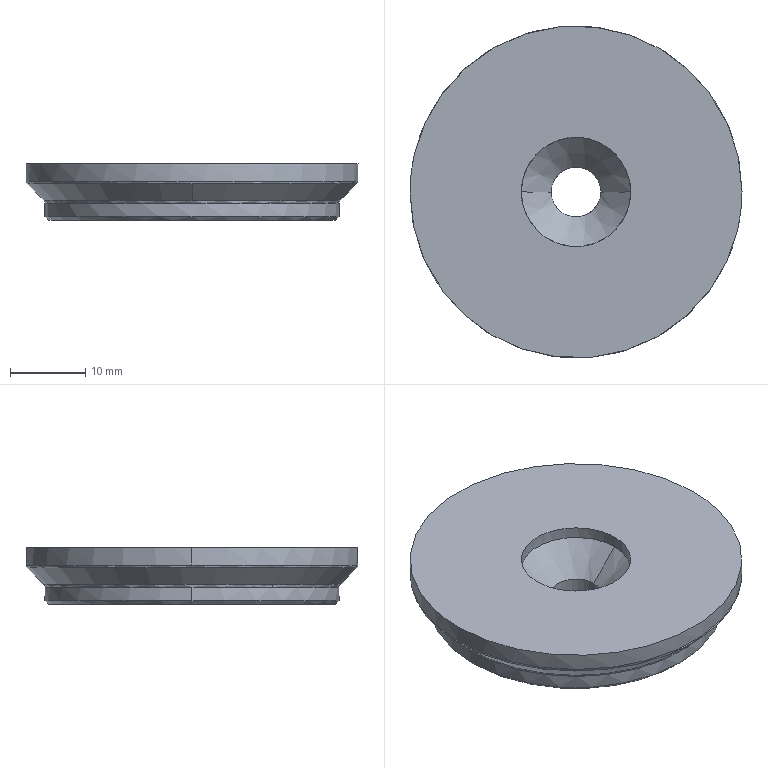Part | STEP file | Suporte_1-A | 1 solid | 20 faces | box 44 x 44 x 7.51 mm | volume 9486 mm3 | cylinder 8 | cone 6 | spline 4 | plane 2 | commonest cylinder face diameters 6.6 x2 14.5 x2 39 x2 44 x2